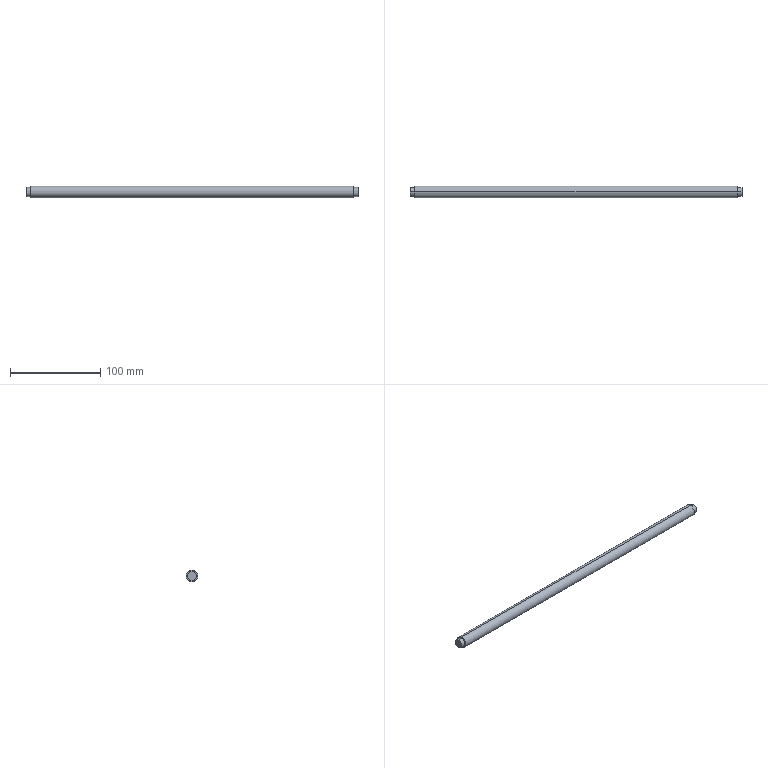Part | SolidWorks | features ICE 4, Chamfer 1, Extrusion 1, Helix 1, SweepCut 1 | 1 solid | 10 faces | box 367 x 13 x 13 mm | volume 48171 mm3 | cylinder 6 | plane 4 | commonest cylinder face diameters 10 x4 13 x2
STEP:
#1=CARTESIAN_POINT('',(-183.5,0.,5.));
#2=VERTEX_POINT('',#1);
#3=CARTESIAN_POINT('',(-183.5,0.,-5.));
#4=VERTEX_POINT('',#3);
#5=CARTESIAN_POINT('',(-183.5,0.,0.));
#6=DIRECTION('',(-1.,0.,0.));
#7=DIRECTION('',(0.,0.,1.));
#8=AXIS2_PLACEMENT_3D('',#5,#6,#7);
#9=CIRCLE('',#8,5.);
#10=EDGE_CURVE('',#2,#4,#9,.T.);
#11=ORIENTED_EDGE('',*,*,#10,.F.);
#12=CARTESIAN_POINT('',(-178.5,0.,5.));
#13=VERTEX_POINT('',#12);
#14=CARTESIAN_POINT('',(-183.5,0.,5.));
#15=DIRECTION('',(1.,0.,0.));
#16=VECTOR('',#15,1000.);
#17=LINE('',#14,#16);
#18=EDGE_CURVE('',#2,#13,#17,.T.);
#19=ORIENTED_EDGE('',*,*,#18,.T.);
#20=CARTESIAN_POINT('',(-178.5,0.,-5.));
#21=VERTEX_POINT('',#20);
#22=CARTESIAN_POINT('',(-178.5,0.,0.));
#23=DIRECTION('',(-1.,0.,0.));
#24=DIRECTION('',(0.,0.,1.));
#25=AXIS2_PLACEMENT_3D('',#22,#23,#24);
#26=CIRCLE('',#25,5.);
#27=EDGE_CURVE('',#13,#21,#26,.T.);
#28=ORIENTED_EDGE('',*,*,#27,.T.);
#29=CARTESIAN_POINT('',(-183.5,0.,-5.));
#30=DIRECTION('',(1.,0.,0.));
#31=VECTOR('',#30,1000.);
#32=LINE('',#29,#31);
#33=EDGE_CURVE('',#4,#21,#32,.T.);
#34=ORIENTED_EDGE('',*,*,#33,.F.);
#35=EDGE_LOOP('',(#11,#19,#28,#34));
#36=FACE_OUTER_BOUND('',#35,.T.);
#37=CARTESIAN_POINT('',(-183.5,0.,0.));
#38=DIRECTION('',(1.,0.,0.));
#39=DIRECTION('',(0.,0.,-1.));
#40=AXIS2_PLACEMENT_3D('',#37,#38,#39);
#41=CYLINDRICAL_SURFACE('',#40,5.);
#42=ADVANCED_FACE('',(#36),#41,.T.);
#43=CARTESIAN_POINT('',(183.5,0.,-5.));
#44=VERTEX_POINT('',#43);
#45=CARTESIAN_POINT('',(183.5,0.,5.));
#46=VERTEX_POINT('',#45);
#47=CARTESIAN_POINT('',(183.5,0.,0.));
#48=DIRECTION('',(1.,0.,0.));
#49=DIRECTION('',(0.,0.,-1.));
#50=AXIS2_PLACEMENT_3D('',#47,#48,#49);
#51=CIRCLE('',#50,5.);
#52=EDGE_CURVE('',#44,#46,#51,.T.);
#53=ORIENTED_EDGE('',*,*,#52,.F.);
#54=CARTESIAN_POINT('',(178.5,0.,-5.));
#55=VERTEX_POINT('',#54);
#56=CARTESIAN_POINT('',(183.5,0.,-5.));
#57=DIRECTION('',(-1.,0.,0.));
#58=VECTOR('',#57,1000.);
#59=LINE('',#56,#58);
#60=EDGE_CURVE('',#44,#55,#59,.T.);
#61=ORIENTED_EDGE('',*,*,#60,.T.);
#62=CARTESIAN_POINT('',(178.5,0.,5.));
#63=VERTEX_POINT('',#62);
#64=CARTESIAN_POINT('',(178.5,0.,0.));
#65=DIRECTION('',(1.,0.,0.));
#66=DIRECTION('',(0.,0.,-1.));
#67=AXIS2_PLACEMENT_3D('',#64,#65,#66);
#68=CIRCLE('',#67,5.);
#69=EDGE_CURVE('',#55,#63,#68,.T.);
#70=ORIENTED_EDGE('',*,*,#69,.T.);
#71=CARTESIAN_POINT('',(183.5,0.,5.));
#72=DIRECTION('',(-1.,0.,0.));
#73=VECTOR('',#72,1000.);
#74=LINE('',#71,#73);
#75=EDGE_CURVE('',#46,#63,#74,.T.);
#76=ORIENTED_EDGE('',*,*,#75,.F.);
#77=EDGE_LOOP('',(#53,#61,#70,#76));
#78=FACE_OUTER_BOUND('',#77,.T.);
#79=CARTESIAN_POINT('',(183.5,0.,0.));
#80=DIRECTION('',(-1.,0.,0.));
#81=DIRECTION('',(0.,0.,1.));
#82=AXIS2_PLACEMENT_3D('',#79,#80,#81);
#83=CYLINDRICAL_SURFACE('',#82,5.);
#84=ADVANCED_FACE('',(#78),#83,.T.);
#85=CARTESIAN_POINT('',(178.5,0.,-6.5));
#86=VERTEX_POINT('',#85);
#87=CARTESIAN_POINT('',(178.5,0.,6.5));
#88=VERTEX_POINT('',#87);
#89=CARTESIAN_POINT('',(178.5,0.,0.));
#90=DIRECTION('',(1.,0.,0.));
#91=DIRECTION('',(0.,0.,-1.));
#92=AXIS2_PLACEMENT_3D('',#89,#90,#91);
#93=CIRCLE('',#92,6.5);
#94=EDGE_CURVE('',#86,#88,#93,.T.);
#95=ORIENTED_EDGE('',*,*,#94,.F.);
#96=CARTESIAN_POINT('',(-178.5,0.,-6.5));
#97=VERTEX_POINT('',#96);
#98=CARTESIAN_POINT('',(178.5,0.,-6.5));
#99=DIRECTION('',(-1.,0.,0.));
#100=VECTOR('',#99,1000.);
#101=LINE('',#98,#100);
#102=EDGE_CURVE('',#86,#97,#101,.T.);
#103=ORIENTED_EDGE('',*,*,#102,.T.);
#104=CARTESIAN_POINT('',(-178.5,0.,6.5));
#105=VERTEX_POINT('',#104);
#106=CARTESIAN_POINT('',(-178.5,0.,0.));
#107=DIRECTION('',(1.,0.,0.));
#108=DIRECTION('',(0.,0.,-1.));
#109=AXIS2_PLACEMENT_3D('',#106,#107,#108);
#110=CIRCLE('',#109,6.5);
#111=EDGE_CURVE('',#97,#105,#110,.T.);
#112=ORIENTED_EDGE('',*,*,#111,.T.);
#113=CARTESIAN_POINT('',(178.5,0.,6.5));
#114=DIRECTION('',(-1.,0.,0.));
#115=VECTOR('',#114,1000.);
#116=LINE('',#113,#115);
#117=EDGE_CURVE('',#88,#105,#116,.T.);
#118=ORIENTED_EDGE('',*,*,#117,.F.);
#119=EDGE_LOOP('',(#95,#103,#112,#118));
#120=FACE_OUTER_BOUND('',#119,.T.);
#121=CARTESIAN_POINT('',(178.5,0.,0.));
#122=DIRECTION('',(-1.,0.,0.));
#123=DIRECTION('',(0.,0.,1.));
#124=AXIS2_PLACEMENT_3D('',#121,#122,#123);
#125=CYLINDRICAL_SURFACE('',#124,6.5);
#126=ADVANCED_FACE('',(#120),#125,.T.);
#127=ORIENTED_EDGE('',*,*,#102,.F.);
#128=CARTESIAN_POINT('',(178.5,0.,0.));
#129=DIRECTION('',(1.,0.,0.));
#130=DIRECTION('',(0.,0.,-1.));
#131=AXIS2_PLACEMENT_3D('',#128,#129,#130);
#132=CIRCLE('',#131,6.5);
#133=EDGE_CURVE('',#88,#86,#132,.T.);
#134=ORIENTED_EDGE('',*,*,#133,.F.);
#135=ORIENTED_EDGE('',*,*,#117,.T.);
#136=CARTESIAN_POINT('',(-178.5,0.,0.));
#137=DIRECTION('',(1.,0.,0.));
#138=DIRECTION('',(0.,0.,-1.));
#139=AXIS2_PLACEMENT_3D('',#136,#137,#138);
#140=CIRCLE('',#139,6.5);
#141=EDGE_CURVE('',#105,#97,#140,.T.);
#142=ORIENTED_EDGE('',*,*,#141,.T.);
#143=EDGE_LOOP('',(#127,#134,#135,#142));
#144=FACE_OUTER_BOUND('',#143,.T.);
#145=CARTESIAN_POINT('',(178.5,0.,0.));
#146=DIRECTION('',(-1.,0.,0.));
#147=DIRECTION('',(0.,0.,1.));
#148=AXIS2_PLACEMENT_3D('',#145,#146,#147);
#149=CYLINDRICAL_SURFACE('',#148,6.5);
#150=ADVANCED_FACE('',(#144),#149,.T.);
#151=CARTESIAN_POINT('',(178.5,0.,0.));
#152=DIRECTION('',(1.,0.,0.));
#153=DIRECTION('',(0.,0.,-1.));
#154=AXIS2_PLACEMENT_3D('',#151,#152,#153);
#155=CIRCLE('',#154,5.);
#156=EDGE_CURVE('',#63,#55,#155,.T.);
#157=ORIENTED_EDGE('',*,*,#156,.F.);
#158=ORIENTED_EDGE('',*,*,#69,.F.);
#159=EDGE_LOOP('',(#157,#158));
#160=FACE_BOUND('',#159,.T.);
#161=ORIENTED_EDGE('',*,*,#133,.T.);
#162=ORIENTED_EDGE('',*,*,#94,.T.);
#163=EDGE_LOOP('',(#161,#162));
#164=FACE_OUTER_BOUND('',#163,.T.);
#165=CARTESIAN_POINT('',(178.5,0.,0.));
#166=DIRECTION('',(1.,0.,0.));
#167=DIRECTION('',(0.,0.,-1.));
#168=AXIS2_PLACEMENT_3D('',#165,#166,#167);
#169=PLANE('',#168);
#170=ADVANCED_FACE('',(#160,#164),#169,.T.);
#171=CARTESIAN_POINT('',(-178.5,0.,0.));
#172=DIRECTION('',(-1.,0.,0.));
#173=DIRECTION('',(0.,0.,1.));
#174=AXIS2_PLACEMENT_3D('',#171,#172,#173);
#175=CIRCLE('',#174,5.);
#176=EDGE_CURVE('',#21,#13,#175,.T.);
#177=ORIENTED_EDGE('',*,*,#176,.F.);
#178=ORIENTED_EDGE('',*,*,#27,.F.);
#179=EDGE_LOOP('',(#177,#178));
#180=FACE_BOUND('',#179,.T.);
#181=ORIENTED_EDGE('',*,*,#141,.F.);
#182=ORIENTED_EDGE('',*,*,#111,.F.);
#183=EDGE_LOOP('',(#181,#182));
#184=FACE_OUTER_BOUND('',#183,.T.);
#185=CARTESIAN_POINT('',(-178.5,0.,0.));
#186=DIRECTION('',(1.,0.,0.));
#187=DIRECTION('',(0.,0.,-1.));
#188=AXIS2_PLACEMENT_3D('',#185,#186,#187);
#189=PLANE('',#188);
#190=ADVANCED_FACE('',(#180,#184),#189,.F.);
#191=ORIENTED_EDGE('',*,*,#60,.F.);
#192=CARTESIAN_POINT('',(183.5,0.,0.));
#193=DIRECTION('',(1.,0.,0.));
#194=DIRECTION('',(0.,0.,-1.));
#195=AXIS2_PLACEMENT_3D('',#192,#193,#194);
#196=CIRCLE('',#195,5.);
#197=EDGE_CURVE('',#46,#44,#196,.T.);
#198=ORIENTED_EDGE('',*,*,#197,.F.);
#199=ORIENTED_EDGE('',*,*,#75,.T.);
#200=ORIENTED_EDGE('',*,*,#156,.T.);
#201=EDGE_LOOP('',(#191,#198,#199,#200));
#202=FACE_OUTER_BOUND('',#201,.T.);
#203=CARTESIAN_POINT('',(183.5,0.,0.));
#204=DIRECTION('',(-1.,0.,0.));
#205=DIRECTION('',(0.,0.,1.));
#206=AXIS2_PLACEMENT_3D('',#203,#204,#205);
#207=CYLINDRICAL_SURFACE('',#206,5.);
#208=ADVANCED_FACE('',(#202),#207,.T.);
#209=ORIENTED_EDGE('',*,*,#197,.T.);
#210=ORIENTED_EDGE('',*,*,#52,.T.);
#211=EDGE_LOOP('',(#209,#210));
#212=FACE_OUTER_BOUND('',#211,.T.);
#213=CARTESIAN_POINT('',(183.5,0.,0.));
#214=DIRECTION('',(1.,0.,0.));
#215=DIRECTION('',(0.,0.,-1.));
#216=AXIS2_PLACEMENT_3D('',#213,#214,#215);
#217=PLANE('',#216);
#218=ADVANCED_FACE('',(#212),#217,.T.);
#219=ORIENTED_EDGE('',*,*,#18,.F.);
#220=CARTESIAN_POINT('',(-183.5,0.,0.));
#221=DIRECTION('',(-1.,0.,0.));
#222=DIRECTION('',(0.,0.,1.));
#223=AXIS2_PLACEMENT_3D('',#220,#221,#222);
#224=CIRCLE('',#223,5.);
#225=EDGE_CURVE('',#4,#2,#224,.T.);
#226=ORIENTED_EDGE('',*,*,#225,.F.);
#227=ORIENTED_EDGE('',*,*,#33,.T.);
#228=ORIENTED_EDGE('',*,*,#176,.T.);
#229=EDGE_LOOP('',(#219,#226,#227,#228));
#230=FACE_OUTER_BOUND('',#229,.T.);
#231=CARTESIAN_POINT('',(-183.5,0.,0.));
#232=DIRECTION('',(1.,0.,0.));
#233=DIRECTION('',(0.,0.,-1.));
#234=AXIS2_PLACEMENT_3D('',#231,#232,#233);
#235=CYLINDRICAL_SURFACE('',#234,5.);
#236=ADVANCED_FACE('',(#230),#235,.T.);
#237=ORIENTED_EDGE('',*,*,#225,.T.);
#238=ORIENTED_EDGE('',*,*,#10,.T.);
#239=EDGE_LOOP('',(#237,#238));
#240=FACE_OUTER_BOUND('',#239,.T.);
#241=CARTESIAN_POINT('',(-183.5,0.,0.));
#242=DIRECTION('',(-1.,0.,0.));
#243=DIRECTION('',(0.,0.,1.));
#244=AXIS2_PLACEMENT_3D('',#241,#242,#243);
#245=PLANE('',#244);
#246=ADVANCED_FACE('',(#240),#245,.T.);
#247=CLOSED_SHELL('',(#42,#84,#126,#150,#170,#190,#208,#218,#236,#246));
#248=MANIFOLD_SOLID_BREP('',#247);
#249=CARTESIAN_POINT('',(0.,0.,0.));
#250=DIRECTION('',(0.,0.,1.));
#251=DIRECTION('',(1.,0.,0.));
#252=AXIS2_PLACEMENT_3D('',#249,#250,#251);
#253=(LENGTH_UNIT()NAMED_UNIT(*)SI_UNIT(.MILLI.,.METRE.));
#254=UNCERTAINTY_MEASURE_WITH_UNIT(LENGTH_MEASURE(0.00001),#253,'','');
#255=(NAMED_UNIT(*)PLANE_ANGLE_UNIT()SI_UNIT($,.RADIAN.));
#256=(NAMED_UNIT(*)SI_UNIT($,.STERADIAN.)SOLID_ANGLE_UNIT());
#257=(GEOMETRIC_REPRESENTATION_CONTEXT(3)GLOBAL_UNCERTAINTY_ASSIGNED_CONTEXT((#254))GLOBAL_UNIT_ASSIGNED_CONTEXT((#253,#255,#256))REPRESENTATION_CONTEXT('',''));
#258=ADVANCED_BREP_SHAPE_REPRESENTATION('',(#248,#252),#257);